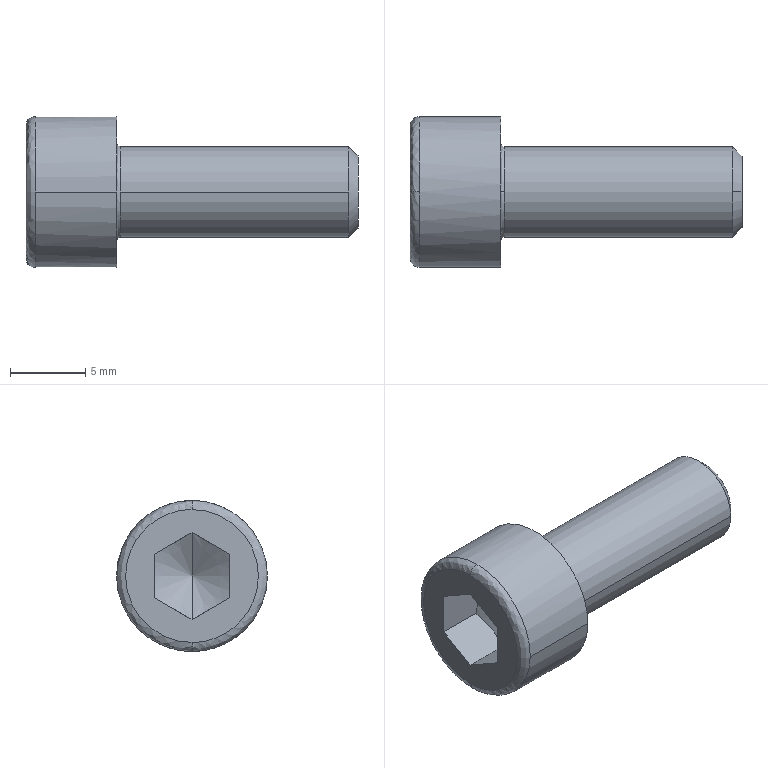Part | STEP file | Broached Socket Head Cap Screw - Metric M6x1 x 16 | 1 solid | 21 faces | box 22 x 10 x 10 mm | volume 839.144 mm3 | plane 9 | spline 4 | cylinder 4 | cone 4 | commonest cylinder face diameters 6 x2 10 x2